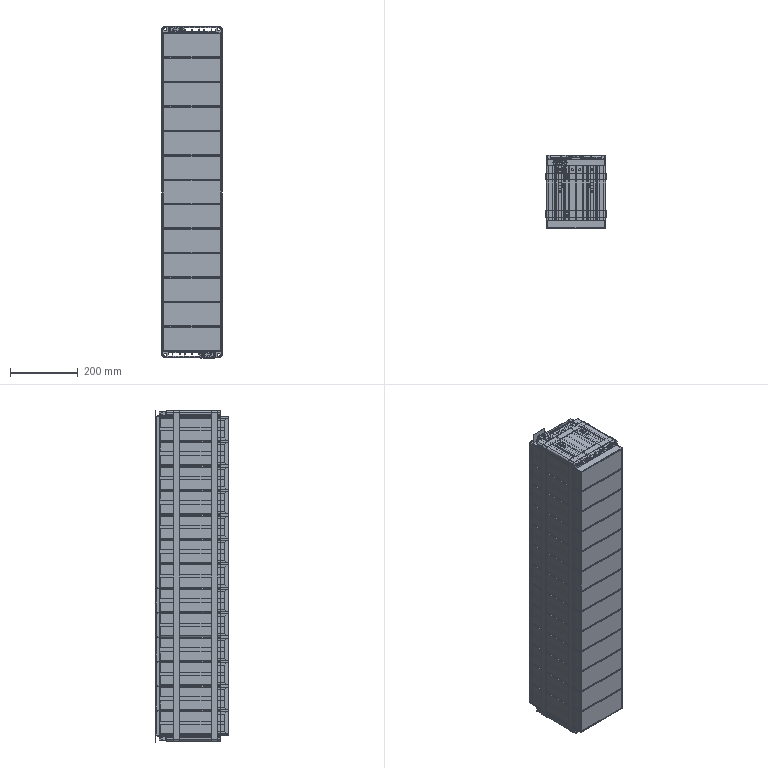Part | NX | features BREP 16 | 76 solids | 12831 faces | volume 34773936 mm3 | plane 7794 | cylinder 4710 | cone 159 | torus 76 | spline 64 | sphere 28 | commonest cylinder face diameters 8 x996 2 x605 6 x442 4 x406 0.4 x236 3 x208